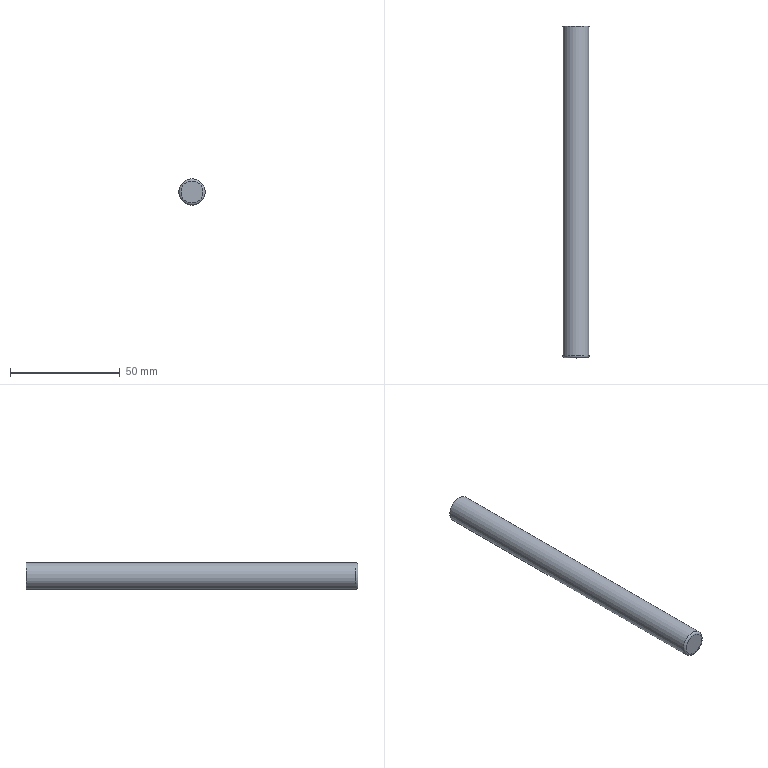Part | STEP file | Tube necking machine_id14_x_t | 1 solid | 4 faces | box 12 x 151.5 x 12 mm | volume 17126 mm3 | plane 2 | cylinder 1 | torus 1 | commonest cylinder face diameters 12 x1
STEP:
#1=CARTESIAN_POINT('',(0.,0.,0.));
#2=DIRECTION('',(0.,0.,1.));
#3=DIRECTION('',(1.,0.,0.));
#4=AXIS2_PLACEMENT_3D('',#1,#2,#3);
#5=CARTESIAN_POINT('',(26.5,-259.,183.));
#6=VERTEX_POINT('',#5);
#7=CARTESIAN_POINT('',(26.5,-259.,195.));
#8=VERTEX_POINT('',#7);
#9=CARTESIAN_POINT('',(26.5,-259.,189.));
#10=DIRECTION('',(0.,1.,0.));
#11=DIRECTION('',(0.,0.,-1.));
#12=AXIS2_PLACEMENT_3D('',#9,#10,#11);
#13=CIRCLE('',#12,6.);
#14=CARTESIAN_POINT('',(0.,-259.,0.));
#15=DIRECTION('',(0.,-1.,0.));
#16=DIRECTION('',(0.,0.,-1.));
#17=AXIS2_PLACEMENT_3D('',#14,#15,#16);
#18=PLANE('',#17);
#19=CARTESIAN_POINT('',(-183.,26.5));
#20=CARTESIAN_POINT('',(-183.,16.108));
#21=CARTESIAN_POINT('',(-192.,21.304));
#22=CARTESIAN_POINT('',(-201.,26.5));
#23=CARTESIAN_POINT('',(-192.,31.696));
#24=CARTESIAN_POINT('',(-183.,36.892));
#25=CARTESIAN_POINT('',(-183.,26.5));
#26=(BOUNDED_CURVE()B_SPLINE_CURVE(2,(#19,#20,#21,#22,#23,#24,#25),.UNSPECIFIED.,.T.,.F.)B_SPLINE_CURVE_WITH_KNOTS((1,2,2,2,2,1),(-2.094,0.,2.094,4.189,6.283,8.378),.UNSPECIFIED.)CURVE()GEOMETRIC_REPRESENTATION_ITEM()RATIONAL_B_SPLINE_CURVE((1.,0.5,1.,0.5,1.,0.5,1.))REPRESENTATION_ITEM(''));
#27=(GEOMETRIC_REPRESENTATION_CONTEXT(2)PARAMETRIC_REPRESENTATION_CONTEXT()REPRESENTATION_CONTEXT('',''));
#28=DEFINITIONAL_REPRESENTATION('',(#26),#27);
#29=PCURVE('',#18,#28);
#30=CARTESIAN_POINT('',(26.5,-807.,189.));
#31=DIRECTION('',(0.,1.,0.));
#32=DIRECTION('',(0.,0.,1.));
#33=AXIS2_PLACEMENT_3D('',#30,#31,#32);
#34=CYLINDRICAL_SURFACE('',#33,6.);
#35=CARTESIAN_POINT('',(3.142,548.));
#36=DIRECTION('',(1.,0.));
#37=VECTOR('',#36,1.);
#38=LINE('',#35,#37);
#39=(GEOMETRIC_REPRESENTATION_CONTEXT(2)PARAMETRIC_REPRESENTATION_CONTEXT()REPRESENTATION_CONTEXT('',''));
#40=DEFINITIONAL_REPRESENTATION('',(#38),#39);
#41=PCURVE('',#34,#40);
#42=SURFACE_CURVE('',#13,(#29,#41),.PCURVE_S1.);
#43=EDGE_CURVE('',#6,#8,#42,.T.);
#44=ORIENTED_EDGE('',*,*,#43,.T.);
#45=CARTESIAN_POINT('',(26.5,-259.,189.));
#46=DIRECTION('',(0.,1.,0.));
#47=DIRECTION('',(0.,0.,-1.));
#48=AXIS2_PLACEMENT_3D('',#45,#46,#47);
#49=CIRCLE('',#48,6.);
#50=CARTESIAN_POINT('',(-183.,26.5));
#51=CARTESIAN_POINT('',(-183.,16.108));
#52=CARTESIAN_POINT('',(-192.,21.304));
#53=CARTESIAN_POINT('',(-201.,26.5));
#54=CARTESIAN_POINT('',(-192.,31.696));
#55=CARTESIAN_POINT('',(-183.,36.892));
#56=CARTESIAN_POINT('',(-183.,26.5));
#57=(BOUNDED_CURVE()B_SPLINE_CURVE(2,(#50,#51,#52,#53,#54,#55,#56),.UNSPECIFIED.,.T.,.F.)B_SPLINE_CURVE_WITH_KNOTS((1,2,2,2,2,1),(-2.094,0.,2.094,4.189,6.283,8.378),.UNSPECIFIED.)CURVE()GEOMETRIC_REPRESENTATION_ITEM()RATIONAL_B_SPLINE_CURVE((1.,0.5,1.,0.5,1.,0.5,1.))REPRESENTATION_ITEM(''));
#58=(GEOMETRIC_REPRESENTATION_CONTEXT(2)PARAMETRIC_REPRESENTATION_CONTEXT()REPRESENTATION_CONTEXT('',''));
#59=DEFINITIONAL_REPRESENTATION('',(#57),#58);
#60=PCURVE('',#18,#59);
#61=CARTESIAN_POINT('',(-3.142,548.));
#62=DIRECTION('',(1.,0.));
#63=VECTOR('',#62,1.);
#64=LINE('',#61,#63);
#65=(GEOMETRIC_REPRESENTATION_CONTEXT(2)PARAMETRIC_REPRESENTATION_CONTEXT()REPRESENTATION_CONTEXT('',''));
#66=DEFINITIONAL_REPRESENTATION('',(#64),#65);
#67=PCURVE('',#34,#66);
#68=SURFACE_CURVE('',#49,(#60,#67),.PCURVE_S1.);
#69=EDGE_CURVE('',#8,#6,#68,.T.);
#70=ORIENTED_EDGE('',*,*,#69,.T.);
#71=EDGE_LOOP('',(#44,#70));
#72=FACE_BOUND('',#71,.T.);
#73=ADVANCED_FACE('',(#72),#18,.F.);
#74=ORIENTED_EDGE('',*,*,#69,.F.);
#75=CARTESIAN_POINT('',(26.5,-409.5,195.));
#76=VERTEX_POINT('',#75);
#77=CARTESIAN_POINT('',(26.5,-409.5,195.));
#78=CARTESIAN_POINT('',(26.5,-259.,195.));
#79=B_SPLINE_CURVE_WITH_KNOTS('',1,(#77,#78),.UNSPECIFIED.,.F.,.F.,(2,2),(397.5,548.),.PIECEWISE_BEZIER_KNOTS.);
#80=CARTESIAN_POINT('',(0.,0.));
#81=DIRECTION('',(0.,1.));
#82=VECTOR('',#81,1.);
#83=LINE('',#80,#82);
#84=(GEOMETRIC_REPRESENTATION_CONTEXT(2)PARAMETRIC_REPRESENTATION_CONTEXT()REPRESENTATION_CONTEXT('',''));
#85=DEFINITIONAL_REPRESENTATION('',(#83),#84);
#86=PCURVE('',#34,#85);
#87=CARTESIAN_POINT('',(6.283,0.));
#88=DIRECTION('',(0.,1.));
#89=VECTOR('',#88,1.);
#90=LINE('',#87,#89);
#91=(GEOMETRIC_REPRESENTATION_CONTEXT(2)PARAMETRIC_REPRESENTATION_CONTEXT()REPRESENTATION_CONTEXT('',''));
#92=DEFINITIONAL_REPRESENTATION('',(#90),#91);
#93=PCURVE('',#34,#92);
#94=SEAM_CURVE('',#79,(#86,#93),.PCURVE_S1.);
#95=EDGE_CURVE('',#76,#8,#94,.T.);
#96=ORIENTED_EDGE('',*,*,#95,.F.);
#97=CARTESIAN_POINT('',(26.5,-409.5,189.));
#98=DIRECTION('',(0.,1.,0.));
#99=DIRECTION('',(0.,0.,1.));
#100=AXIS2_PLACEMENT_3D('',#97,#98,#99);
#101=CIRCLE('',#100,6.);
#102=CARTESIAN_POINT('',(0.,397.5));
#103=DIRECTION('',(1.,0.));
#104=VECTOR('',#103,1.);
#105=LINE('',#102,#104);
#106=(GEOMETRIC_REPRESENTATION_CONTEXT(2)PARAMETRIC_REPRESENTATION_CONTEXT()REPRESENTATION_CONTEXT('',''));
#107=DEFINITIONAL_REPRESENTATION('',(#105),#106);
#108=PCURVE('',#34,#107);
#109=CARTESIAN_POINT('',(26.5,-409.5,189.));
#110=DIRECTION('',(0.,1.,0.));
#111=DIRECTION('',(0.,0.,1.));
#112=AXIS2_PLACEMENT_3D('',#109,#110,#111);
#113=TOROIDAL_SURFACE('',#112,5.,1.);
#114=CARTESIAN_POINT('',(0.,6.283));
#115=DIRECTION('',(1.,0.));
#116=VECTOR('',#115,1.);
#117=LINE('',#114,#116);
#118=(GEOMETRIC_REPRESENTATION_CONTEXT(2)PARAMETRIC_REPRESENTATION_CONTEXT()REPRESENTATION_CONTEXT('',''));
#119=DEFINITIONAL_REPRESENTATION('',(#117),#118);
#120=PCURVE('',#113,#119);
#121=SURFACE_CURVE('',#101,(#108,#120),.PCURVE_S1.);
#122=EDGE_CURVE('',#76,#76,#121,.T.);
#123=ORIENTED_EDGE('',*,*,#122,.T.);
#124=ORIENTED_EDGE('',*,*,#95,.T.);
#125=ORIENTED_EDGE('',*,*,#43,.F.);
#126=EDGE_LOOP('',(#74,#96,#123,#124,#125));
#127=FACE_BOUND('',#126,.T.);
#128=ADVANCED_FACE('',(#127),#34,.T.);
#129=CARTESIAN_POINT('',(26.5,-410.5,194.));
#130=VERTEX_POINT('',#129);
#131=CARTESIAN_POINT('',(26.5,-410.5,189.));
#132=DIRECTION('',(0.,-1.,0.));
#133=DIRECTION('',(0.,0.,1.));
#134=AXIS2_PLACEMENT_3D('',#131,#132,#133);
#135=CIRCLE('',#134,5.);
#136=CARTESIAN_POINT('',(26.5,-410.5,189.));
#137=DIRECTION('',(0.,1.,0.));
#138=DIRECTION('',(0.,0.,1.));
#139=AXIS2_PLACEMENT_3D('',#136,#137,#138);
#140=PLANE('',#139);
#141=CARTESIAN_POINT('',(5.,0.));
#142=CARTESIAN_POINT('',(5.,-8.66));
#143=CARTESIAN_POINT('',(-2.5,-4.33));
#144=CARTESIAN_POINT('',(-10.,0.));
#145=CARTESIAN_POINT('',(-2.5,4.33));
#146=CARTESIAN_POINT('',(5.,8.66));
#147=CARTESIAN_POINT('',(5.,0.));
#148=(BOUNDED_CURVE()B_SPLINE_CURVE(2,(#141,#142,#143,#144,#145,#146,#147),.UNSPECIFIED.,.T.,.F.)B_SPLINE_CURVE_WITH_KNOTS((1,2,2,2,2,1),(-2.094,0.,2.094,4.189,6.283,8.378),.UNSPECIFIED.)CURVE()GEOMETRIC_REPRESENTATION_ITEM()RATIONAL_B_SPLINE_CURVE((1.,0.5,1.,0.5,1.,0.5,1.))REPRESENTATION_ITEM(''));
#149=(GEOMETRIC_REPRESENTATION_CONTEXT(2)PARAMETRIC_REPRESENTATION_CONTEXT()REPRESENTATION_CONTEXT('',''));
#150=DEFINITIONAL_REPRESENTATION('',(#148),#149);
#151=PCURVE('',#140,#150);
#152=CARTESIAN_POINT('',(6.283,4.712));
#153=DIRECTION('',(-1.,0.));
#154=VECTOR('',#153,1.);
#155=LINE('',#152,#154);
#156=(GEOMETRIC_REPRESENTATION_CONTEXT(2)PARAMETRIC_REPRESENTATION_CONTEXT()REPRESENTATION_CONTEXT('',''));
#157=DEFINITIONAL_REPRESENTATION('',(#155),#156);
#158=PCURVE('',#113,#157);
#159=SURFACE_CURVE('',#135,(#151,#158),.PCURVE_S1.);
#160=EDGE_CURVE('',#130,#130,#159,.T.);
#161=ORIENTED_EDGE('',*,*,#160,.T.);
#162=EDGE_LOOP('',(#161));
#163=FACE_BOUND('',#162,.T.);
#164=ADVANCED_FACE('',(#163),#140,.F.);
#165=ORIENTED_EDGE('',*,*,#160,.F.);
#166=CARTESIAN_POINT('',(26.5,-410.5,194.));
#167=CARTESIAN_POINT('',(26.5,-410.5,194.267));
#168=CARTESIAN_POINT('',(26.5,-410.415,194.528));
#169=CARTESIAN_POINT('',(26.5,-410.252,194.752));
#170=CARTESIAN_POINT('',(26.5,-410.028,194.915));
#171=CARTESIAN_POINT('',(26.5,-409.767,195.));
#172=CARTESIAN_POINT('',(26.5,-409.5,195.));
#173=(BOUNDED_CURVE()B_SPLINE_CURVE(6,(#166,#167,#168,#169,#170,#171,#172),.UNSPECIFIED.,.F.,.F.)B_SPLINE_CURVE_WITH_KNOTS((7,7),(4.712,6.283),.PIECEWISE_BEZIER_KNOTS.)CURVE()GEOMETRIC_REPRESENTATION_ITEM()RATIONAL_B_SPLINE_CURVE((1.031,1.01,0.9979,0.994,0.9979,1.01,1.031))REPRESENTATION_ITEM(''));
#174=CARTESIAN_POINT('',(6.283,0.));
#175=DIRECTION('',(0.,1.));
#176=VECTOR('',#175,1.);
#177=LINE('',#174,#176);
#178=(GEOMETRIC_REPRESENTATION_CONTEXT(2)PARAMETRIC_REPRESENTATION_CONTEXT()REPRESENTATION_CONTEXT('',''));
#179=DEFINITIONAL_REPRESENTATION('',(#177),#178);
#180=PCURVE('',#113,#179);
#181=CARTESIAN_POINT('',(0.,0.));
#182=DIRECTION('',(0.,1.));
#183=VECTOR('',#182,1.);
#184=LINE('',#181,#183);
#185=(GEOMETRIC_REPRESENTATION_CONTEXT(2)PARAMETRIC_REPRESENTATION_CONTEXT()REPRESENTATION_CONTEXT('',''));
#186=DEFINITIONAL_REPRESENTATION('',(#184),#185);
#187=PCURVE('',#113,#186);
#188=SEAM_CURVE('',#173,(#180,#187),.PCURVE_S1.);
#189=EDGE_CURVE('',#130,#76,#188,.T.);
#190=ORIENTED_EDGE('',*,*,#189,.T.);
#191=ORIENTED_EDGE('',*,*,#122,.F.);
#192=ORIENTED_EDGE('',*,*,#189,.F.);
#193=EDGE_LOOP('',(#165,#190,#191,#192));
#194=FACE_BOUND('',#193,.T.);
#195=ADVANCED_FACE('',(#194),#113,.T.);
#196=CLOSED_SHELL('',(#73,#128,#164,#195));
#197=MANIFOLD_SOLID_BREP('',#196);
#198=(LENGTH_UNIT()NAMED_UNIT(*)SI_UNIT(.MILLI.,.METRE.));
#199=UNCERTAINTY_MEASURE_WITH_UNIT(LENGTH_MEASURE(0.000005),#198,'','');
#200=(NAMED_UNIT(*)PLANE_ANGLE_UNIT()SI_UNIT($,.RADIAN.));
#201=(NAMED_UNIT(*)SI_UNIT($,.STERADIAN.)SOLID_ANGLE_UNIT());
#202=(GEOMETRIC_REPRESENTATION_CONTEXT(3)GLOBAL_UNCERTAINTY_ASSIGNED_CONTEXT((#199))GLOBAL_UNIT_ASSIGNED_CONTEXT((#198,#200,#201))REPRESENTATION_CONTEXT('',''));
#203=ADVANCED_BREP_SHAPE_REPRESENTATION('',(#4,#197),#202);